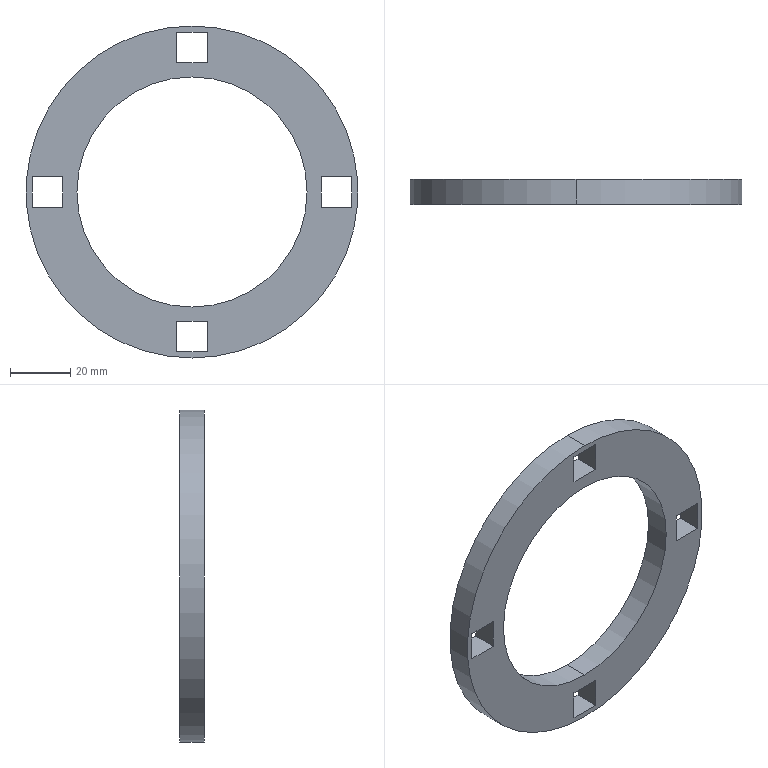Part | SolidWorks | features BaseBody 1 | 1 solid | 22 faces | box 110 x 8.25 x 110 mm | volume 37347 mm3 | plane 18 | cylinder 4 | commonest cylinder face diameters 76.25 x2 110 x2
STEP:
#1=CARTESIAN_POINT('',(-2080.019,753.694,-1572.562));
#2=VERTEX_POINT('',#1);
#3=CARTESIAN_POINT('',(-2090.144,753.694,-1572.562));
#4=VERTEX_POINT('',#3);
#5=CARTESIAN_POINT('',(-2080.019,753.694,-1572.562));
#6=DIRECTION('',(-1.,0.,0.));
#7=VECTOR('',#6,1000.);
#8=LINE('',#5,#7);
#9=EDGE_CURVE('',#2,#4,#8,.T.);
#10=ORIENTED_EDGE('',*,*,#9,.T.);
#11=CARTESIAN_POINT('',(-2090.144,753.694,-1582.687));
#12=VERTEX_POINT('',#11);
#13=CARTESIAN_POINT('',(-2090.144,753.694,-1572.562));
#14=DIRECTION('',(0.,0.,-1.));
#15=VECTOR('',#14,1000.);
#16=LINE('',#13,#15);
#17=EDGE_CURVE('',#4,#12,#16,.T.);
#18=ORIENTED_EDGE('',*,*,#17,.T.);
#19=CARTESIAN_POINT('',(-2080.019,753.694,-1582.687));
#20=VERTEX_POINT('',#19);
#21=CARTESIAN_POINT('',(-2090.144,753.694,-1582.687));
#22=DIRECTION('',(1.,0.,0.));
#23=VECTOR('',#22,1000.);
#24=LINE('',#21,#23);
#25=EDGE_CURVE('',#12,#20,#24,.T.);
#26=ORIENTED_EDGE('',*,*,#25,.T.);
#27=CARTESIAN_POINT('',(-2080.019,753.694,-1582.687));
#28=DIRECTION('',(0.,0.,1.));
#29=VECTOR('',#28,1000.);
#30=LINE('',#27,#29);
#31=EDGE_CURVE('',#20,#2,#30,.T.);
#32=ORIENTED_EDGE('',*,*,#31,.T.);
#33=EDGE_LOOP('',(#10,#18,#26,#32));
#34=FACE_BOUND('',#33,.T.);
#35=CARTESIAN_POINT('',(-2138.012,753.694,-1524.694));
#36=VERTEX_POINT('',#35);
#37=CARTESIAN_POINT('',(-2138.012,753.694,-1534.819));
#38=VERTEX_POINT('',#37);
#39=CARTESIAN_POINT('',(-2138.012,753.694,-1524.694));
#40=DIRECTION('',(0.,0.,-1.));
#41=VECTOR('',#40,1000.);
#42=LINE('',#39,#41);
#43=EDGE_CURVE('',#36,#38,#42,.T.);
#44=ORIENTED_EDGE('',*,*,#43,.T.);
#45=CARTESIAN_POINT('',(-2127.887,753.694,-1534.819));
#46=VERTEX_POINT('',#45);
#47=CARTESIAN_POINT('',(-2138.012,753.694,-1534.819));
#48=DIRECTION('',(1.,0.,0.));
#49=VECTOR('',#48,1000.);
#50=LINE('',#47,#49);
#51=EDGE_CURVE('',#38,#46,#50,.T.);
#52=ORIENTED_EDGE('',*,*,#51,.T.);
#53=CARTESIAN_POINT('',(-2127.887,753.694,-1524.694));
#54=VERTEX_POINT('',#53);
#55=CARTESIAN_POINT('',(-2127.887,753.694,-1534.819));
#56=DIRECTION('',(0.,0.,1.));
#57=VECTOR('',#56,1000.);
#58=LINE('',#55,#57);
#59=EDGE_CURVE('',#46,#54,#58,.T.);
#60=ORIENTED_EDGE('',*,*,#59,.T.);
#61=CARTESIAN_POINT('',(-2127.887,753.694,-1524.694));
#62=DIRECTION('',(-1.,0.,0.));
#63=VECTOR('',#62,1000.);
#64=LINE('',#61,#63);
#65=EDGE_CURVE('',#54,#36,#64,.T.);
#66=ORIENTED_EDGE('',*,*,#65,.T.);
#67=EDGE_LOOP('',(#44,#52,#60,#66));
#68=FACE_BOUND('',#67,.T.);
#69=CARTESIAN_POINT('',(-2185.88,753.694,-1582.687));
#70=VERTEX_POINT('',#69);
#71=CARTESIAN_POINT('',(-2175.755,753.694,-1582.687));
#72=VERTEX_POINT('',#71);
#73=CARTESIAN_POINT('',(-2185.88,753.694,-1582.687));
#74=DIRECTION('',(1.,0.,0.));
#75=VECTOR('',#74,1000.);
#76=LINE('',#73,#75);
#77=EDGE_CURVE('',#70,#72,#76,.T.);
#78=ORIENTED_EDGE('',*,*,#77,.T.);
#79=CARTESIAN_POINT('',(-2175.755,753.694,-1572.562));
#80=VERTEX_POINT('',#79);
#81=CARTESIAN_POINT('',(-2175.755,753.694,-1582.687));
#82=DIRECTION('',(0.,0.,1.));
#83=VECTOR('',#82,1000.);
#84=LINE('',#81,#83);
#85=EDGE_CURVE('',#72,#80,#84,.T.);
#86=ORIENTED_EDGE('',*,*,#85,.T.);
#87=CARTESIAN_POINT('',(-2185.88,753.694,-1572.562));
#88=VERTEX_POINT('',#87);
#89=CARTESIAN_POINT('',(-2175.755,753.694,-1572.562));
#90=DIRECTION('',(-1.,0.,0.));
#91=VECTOR('',#90,1000.);
#92=LINE('',#89,#91);
#93=EDGE_CURVE('',#80,#88,#92,.T.);
#94=ORIENTED_EDGE('',*,*,#93,.T.);
#95=CARTESIAN_POINT('',(-2185.88,753.694,-1572.562));
#96=DIRECTION('',(0.,0.,-1.));
#97=VECTOR('',#96,1000.);
#98=LINE('',#95,#97);
#99=EDGE_CURVE('',#88,#70,#98,.T.);
#100=ORIENTED_EDGE('',*,*,#99,.T.);
#101=EDGE_LOOP('',(#78,#86,#94,#100));
#102=FACE_BOUND('',#101,.T.);
#103=CARTESIAN_POINT('',(-2127.887,753.694,-1630.555));
#104=VERTEX_POINT('',#103);
#105=CARTESIAN_POINT('',(-2127.887,753.694,-1620.43));
#106=VERTEX_POINT('',#105);
#107=CARTESIAN_POINT('',(-2127.887,753.694,-1630.555));
#108=DIRECTION('',(0.,0.,1.));
#109=VECTOR('',#108,1000.);
#110=LINE('',#107,#109);
#111=EDGE_CURVE('',#104,#106,#110,.T.);
#112=ORIENTED_EDGE('',*,*,#111,.T.);
#113=CARTESIAN_POINT('',(-2138.012,753.694,-1620.43));
#114=VERTEX_POINT('',#113);
#115=CARTESIAN_POINT('',(-2127.887,753.694,-1620.43));
#116=DIRECTION('',(-1.,0.,0.));
#117=VECTOR('',#116,1000.);
#118=LINE('',#115,#117);
#119=EDGE_CURVE('',#106,#114,#118,.T.);
#120=ORIENTED_EDGE('',*,*,#119,.T.);
#121=CARTESIAN_POINT('',(-2138.012,753.694,-1630.555));
#122=VERTEX_POINT('',#121);
#123=CARTESIAN_POINT('',(-2138.012,753.694,-1620.43));
#124=DIRECTION('',(0.,0.,-1.));
#125=VECTOR('',#124,1000.);
#126=LINE('',#123,#125);
#127=EDGE_CURVE('',#114,#122,#126,.T.);
#128=ORIENTED_EDGE('',*,*,#127,.T.);
#129=CARTESIAN_POINT('',(-2138.012,753.694,-1630.555));
#130=DIRECTION('',(1.,0.,0.));
#131=VECTOR('',#130,1000.);
#132=LINE('',#129,#131);
#133=EDGE_CURVE('',#122,#104,#132,.T.);
#134=ORIENTED_EDGE('',*,*,#133,.T.);
#135=EDGE_LOOP('',(#112,#120,#128,#134));
#136=FACE_BOUND('',#135,.T.);
#137=CARTESIAN_POINT('',(-2132.95,753.694,-1539.499));
#138=VERTEX_POINT('',#137);
#139=CARTESIAN_POINT('',(-2132.95,753.694,-1615.749));
#140=VERTEX_POINT('',#139);
#141=CARTESIAN_POINT('',(-2132.95,753.694,-1577.624));
#142=DIRECTION('',(0.,1.,0.));
#143=DIRECTION('',(0.,0.,1.));
#144=AXIS2_PLACEMENT_3D('',#141,#142,#143);
#145=CIRCLE('',#144,38.125);
#146=EDGE_CURVE('',#138,#140,#145,.T.);
#147=ORIENTED_EDGE('',*,*,#146,.F.);
#148=CARTESIAN_POINT('',(-2132.95,753.694,-1577.624));
#149=DIRECTION('',(0.,1.,0.));
#150=DIRECTION('',(0.,0.,-1.));
#151=AXIS2_PLACEMENT_3D('',#148,#149,#150);
#152=CIRCLE('',#151,38.125);
#153=EDGE_CURVE('',#140,#138,#152,.T.);
#154=ORIENTED_EDGE('',*,*,#153,.F.);
#155=EDGE_LOOP('',(#147,#154));
#156=FACE_BOUND('',#155,.T.);
#157=CARTESIAN_POINT('',(-2132.95,753.694,-1632.624));
#158=VERTEX_POINT('',#157);
#159=CARTESIAN_POINT('',(-2132.95,753.694,-1522.624));
#160=VERTEX_POINT('',#159);
#161=CARTESIAN_POINT('',(-2132.95,753.694,-1577.624));
#162=DIRECTION('',(0.,1.,0.));
#163=DIRECTION('',(0.,0.,-1.));
#164=AXIS2_PLACEMENT_3D('',#161,#162,#163);
#165=CIRCLE('',#164,55.);
#166=EDGE_CURVE('',#158,#160,#165,.T.);
#167=ORIENTED_EDGE('',*,*,#166,.T.);
#168=CARTESIAN_POINT('',(-2132.95,753.694,-1577.624));
#169=DIRECTION('',(0.,1.,0.));
#170=DIRECTION('',(0.,0.,1.));
#171=AXIS2_PLACEMENT_3D('',#168,#169,#170);
#172=CIRCLE('',#171,55.);
#173=EDGE_CURVE('',#160,#158,#172,.T.);
#174=ORIENTED_EDGE('',*,*,#173,.T.);
#175=EDGE_LOOP('',(#167,#174));
#176=FACE_OUTER_BOUND('',#175,.T.);
#177=CARTESIAN_POINT('',(-2072.49,753.694,-1517.124));
#178=DIRECTION('',(0.,1.,0.));
#179=DIRECTION('',(1.,0.,0.));
#180=AXIS2_PLACEMENT_3D('',#177,#178,#179);
#181=PLANE('',#180);
#182=ADVANCED_FACE('',(#34,#68,#102,#136,#156,#176),#181,.T.);
#183=CARTESIAN_POINT('',(-2090.144,745.444,-1572.562));
#184=VERTEX_POINT('',#183);
#185=CARTESIAN_POINT('',(-2080.019,745.444,-1572.562));
#186=VERTEX_POINT('',#185);
#187=CARTESIAN_POINT('',(-2090.144,745.444,-1572.562));
#188=DIRECTION('',(1.,0.,0.));
#189=VECTOR('',#188,1000.);
#190=LINE('',#187,#189);
#191=EDGE_CURVE('',#184,#186,#190,.T.);
#192=ORIENTED_EDGE('',*,*,#191,.T.);
#193=CARTESIAN_POINT('',(-2080.019,745.444,-1582.687));
#194=VERTEX_POINT('',#193);
#195=CARTESIAN_POINT('',(-2080.019,745.444,-1572.562));
#196=DIRECTION('',(0.,0.,-1.));
#197=VECTOR('',#196,1000.);
#198=LINE('',#195,#197);
#199=EDGE_CURVE('',#186,#194,#198,.T.);
#200=ORIENTED_EDGE('',*,*,#199,.T.);
#201=CARTESIAN_POINT('',(-2090.144,745.444,-1582.687));
#202=VERTEX_POINT('',#201);
#203=CARTESIAN_POINT('',(-2080.019,745.444,-1582.687));
#204=DIRECTION('',(-1.,0.,0.));
#205=VECTOR('',#204,1000.);
#206=LINE('',#203,#205);
#207=EDGE_CURVE('',#194,#202,#206,.T.);
#208=ORIENTED_EDGE('',*,*,#207,.T.);
#209=CARTESIAN_POINT('',(-2090.144,745.444,-1582.687));
#210=DIRECTION('',(0.,0.,1.));
#211=VECTOR('',#210,1000.);
#212=LINE('',#209,#211);
#213=EDGE_CURVE('',#202,#184,#212,.T.);
#214=ORIENTED_EDGE('',*,*,#213,.T.);
#215=EDGE_LOOP('',(#192,#200,#208,#214));
#216=FACE_BOUND('',#215,.T.);
#217=CARTESIAN_POINT('',(-2138.012,745.444,-1534.819));
#218=VERTEX_POINT('',#217);
#219=CARTESIAN_POINT('',(-2138.012,745.444,-1524.694));
#220=VERTEX_POINT('',#219);
#221=CARTESIAN_POINT('',(-2138.012,745.444,-1534.819));
#222=DIRECTION('',(0.,0.,1.));
#223=VECTOR('',#222,1000.);
#224=LINE('',#221,#223);
#225=EDGE_CURVE('',#218,#220,#224,.T.);
#226=ORIENTED_EDGE('',*,*,#225,.T.);
#227=CARTESIAN_POINT('',(-2127.887,745.444,-1524.694));
#228=VERTEX_POINT('',#227);
#229=CARTESIAN_POINT('',(-2138.012,745.444,-1524.694));
#230=DIRECTION('',(1.,0.,0.));
#231=VECTOR('',#230,1000.);
#232=LINE('',#229,#231);
#233=EDGE_CURVE('',#220,#228,#232,.T.);
#234=ORIENTED_EDGE('',*,*,#233,.T.);
#235=CARTESIAN_POINT('',(-2127.887,745.444,-1534.819));
#236=VERTEX_POINT('',#235);
#237=CARTESIAN_POINT('',(-2127.887,745.444,-1524.694));
#238=DIRECTION('',(0.,0.,-1.));
#239=VECTOR('',#238,1000.);
#240=LINE('',#237,#239);
#241=EDGE_CURVE('',#228,#236,#240,.T.);
#242=ORIENTED_EDGE('',*,*,#241,.T.);
#243=CARTESIAN_POINT('',(-2127.887,745.444,-1534.819));
#244=DIRECTION('',(-1.,0.,0.));
#245=VECTOR('',#244,1000.);
#246=LINE('',#243,#245);
#247=EDGE_CURVE('',#236,#218,#246,.T.);
#248=ORIENTED_EDGE('',*,*,#247,.T.);
#249=EDGE_LOOP('',(#226,#234,#242,#248));
#250=FACE_BOUND('',#249,.T.);
#251=CARTESIAN_POINT('',(-2175.755,745.444,-1582.687));
#252=VERTEX_POINT('',#251);
#253=CARTESIAN_POINT('',(-2185.88,745.444,-1582.687));
#254=VERTEX_POINT('',#253);
#255=CARTESIAN_POINT('',(-2175.755,745.444,-1582.687));
#256=DIRECTION('',(-1.,0.,0.));
#257=VECTOR('',#256,1000.);
#258=LINE('',#255,#257);
#259=EDGE_CURVE('',#252,#254,#258,.T.);
#260=ORIENTED_EDGE('',*,*,#259,.T.);
#261=CARTESIAN_POINT('',(-2185.88,745.444,-1572.562));
#262=VERTEX_POINT('',#261);
#263=CARTESIAN_POINT('',(-2185.88,745.444,-1582.687));
#264=DIRECTION('',(0.,0.,1.));
#265=VECTOR('',#264,1000.);
#266=LINE('',#263,#265);
#267=EDGE_CURVE('',#254,#262,#266,.T.);
#268=ORIENTED_EDGE('',*,*,#267,.T.);
#269=CARTESIAN_POINT('',(-2175.755,745.444,-1572.562));
#270=VERTEX_POINT('',#269);
#271=CARTESIAN_POINT('',(-2185.88,745.444,-1572.562));
#272=DIRECTION('',(1.,0.,0.));
#273=VECTOR('',#272,1000.);
#274=LINE('',#271,#273);
#275=EDGE_CURVE('',#262,#270,#274,.T.);
#276=ORIENTED_EDGE('',*,*,#275,.T.);
#277=CARTESIAN_POINT('',(-2175.755,745.444,-1572.562));
#278=DIRECTION('',(0.,0.,-1.));
#279=VECTOR('',#278,1000.);
#280=LINE('',#277,#279);
#281=EDGE_CURVE('',#270,#252,#280,.T.);
#282=ORIENTED_EDGE('',*,*,#281,.T.);
#283=EDGE_LOOP('',(#260,#268,#276,#282));
#284=FACE_BOUND('',#283,.T.);
#285=CARTESIAN_POINT('',(-2127.887,745.444,-1620.43));
#286=VERTEX_POINT('',#285);
#287=CARTESIAN_POINT('',(-2127.887,745.444,-1630.555));
#288=VERTEX_POINT('',#287);
#289=CARTESIAN_POINT('',(-2127.887,745.444,-1620.43));
#290=DIRECTION('',(0.,0.,-1.));
#291=VECTOR('',#290,1000.);
#292=LINE('',#289,#291);
#293=EDGE_CURVE('',#286,#288,#292,.T.);
#294=ORIENTED_EDGE('',*,*,#293,.T.);
#295=CARTESIAN_POINT('',(-2138.012,745.444,-1630.555));
#296=VERTEX_POINT('',#295);
#297=CARTESIAN_POINT('',(-2127.887,745.444,-1630.555));
#298=DIRECTION('',(-1.,0.,0.));
#299=VECTOR('',#298,1000.);
#300=LINE('',#297,#299);
#301=EDGE_CURVE('',#288,#296,#300,.T.);
#302=ORIENTED_EDGE('',*,*,#301,.T.);
#303=CARTESIAN_POINT('',(-2138.012,745.444,-1620.43));
#304=VERTEX_POINT('',#303);
#305=CARTESIAN_POINT('',(-2138.012,745.444,-1630.555));
#306=DIRECTION('',(0.,0.,1.));
#307=VECTOR('',#306,1000.);
#308=LINE('',#305,#307);
#309=EDGE_CURVE('',#296,#304,#308,.T.);
#310=ORIENTED_EDGE('',*,*,#309,.T.);
#311=CARTESIAN_POINT('',(-2138.012,745.444,-1620.43));
#312=DIRECTION('',(1.,0.,0.));
#313=VECTOR('',#312,1000.);
#314=LINE('',#311,#313);
#315=EDGE_CURVE('',#304,#286,#314,.T.);
#316=ORIENTED_EDGE('',*,*,#315,.T.);
#317=EDGE_LOOP('',(#294,#302,#310,#316));
#318=FACE_BOUND('',#317,.T.);
#319=CARTESIAN_POINT('',(-2132.95,745.444,-1539.499));
#320=VERTEX_POINT('',#319);
#321=CARTESIAN_POINT('',(-2132.95,745.444,-1615.749));
#322=VERTEX_POINT('',#321);
#323=CARTESIAN_POINT('',(-2132.95,745.444,-1577.624));
#324=DIRECTION('',(0.,-1.,0.));
#325=DIRECTION('',(0.,0.,1.));
#326=AXIS2_PLACEMENT_3D('',#323,#324,#325);
#327=CIRCLE('',#326,38.125);
#328=EDGE_CURVE('',#320,#322,#327,.T.);
#329=ORIENTED_EDGE('',*,*,#328,.F.);
#330=CARTESIAN_POINT('',(-2132.95,745.444,-1577.624));
#331=DIRECTION('',(0.,-1.,0.));
#332=DIRECTION('',(0.,0.,-1.));
#333=AXIS2_PLACEMENT_3D('',#330,#331,#332);
#334=CIRCLE('',#333,38.125);
#335=EDGE_CURVE('',#322,#320,#334,.T.);
#336=ORIENTED_EDGE('',*,*,#335,.F.);
#337=EDGE_LOOP('',(#329,#336));
#338=FACE_BOUND('',#337,.T.);
#339=CARTESIAN_POINT('',(-2132.95,745.444,-1632.624));
#340=VERTEX_POINT('',#339);
#341=CARTESIAN_POINT('',(-2132.95,745.444,-1522.624));
#342=VERTEX_POINT('',#341);
#343=CARTESIAN_POINT('',(-2132.95,745.444,-1577.624));
#344=DIRECTION('',(0.,-1.,0.));
#345=DIRECTION('',(0.,0.,-1.));
#346=AXIS2_PLACEMENT_3D('',#343,#344,#345);
#347=CIRCLE('',#346,55.);
#348=EDGE_CURVE('',#340,#342,#347,.T.);
#349=ORIENTED_EDGE('',*,*,#348,.T.);
#350=CARTESIAN_POINT('',(-2132.95,745.444,-1577.624));
#351=DIRECTION('',(0.,-1.,0.));
#352=DIRECTION('',(0.,0.,1.));
#353=AXIS2_PLACEMENT_3D('',#350,#351,#352);
#354=CIRCLE('',#353,55.);
#355=EDGE_CURVE('',#342,#340,#354,.T.);
#356=ORIENTED_EDGE('',*,*,#355,.T.);
#357=EDGE_LOOP('',(#349,#356));
#358=FACE_OUTER_BOUND('',#357,.T.);
#359=CARTESIAN_POINT('',(-2072.49,745.444,-1638.124));
#360=DIRECTION('',(0.,-1.,0.));
#361=DIRECTION('',(0.,0.,-1.));
#362=AXIS2_PLACEMENT_3D('',#359,#360,#361);
#363=PLANE('',#362);
#364=ADVANCED_FACE('',(#216,#250,#284,#318,#338,#358),#363,.T.);
#365=CARTESIAN_POINT('',(-2132.95,745.444,-1632.624));
#366=DIRECTION('',(0.,1.,0.));
#367=VECTOR('',#366,1000.);
#368=LINE('',#365,#367);
#369=EDGE_CURVE('',#340,#158,#368,.T.);
#370=ORIENTED_EDGE('',*,*,#369,.T.);
#371=ORIENTED_EDGE('',*,*,#173,.F.);
#372=CARTESIAN_POINT('',(-2132.95,753.694,-1522.624));
#373=DIRECTION('',(0.,-1.,0.));
#374=VECTOR('',#373,1000.);
#375=LINE('',#372,#374);
#376=EDGE_CURVE('',#160,#342,#375,.T.);
#377=ORIENTED_EDGE('',*,*,#376,.T.);
#378=ORIENTED_EDGE('',*,*,#348,.F.);
#379=EDGE_LOOP('',(#370,#371,#377,#378));
#380=FACE_OUTER_BOUND('',#379,.T.);
#381=CARTESIAN_POINT('',(-2132.95,745.031,-1577.624));
#382=DIRECTION('',(0.,-1.,0.));
#383=DIRECTION('',(-0.08716,0.,-0.9962));
#384=AXIS2_PLACEMENT_3D('',#381,#382,#383);
#385=CYLINDRICAL_SURFACE('',#384,55.);
#386=ADVANCED_FACE('',(#380),#385,.T.);
#387=CARTESIAN_POINT('',(-2132.95,753.694,-1615.749));
#388=DIRECTION('',(0.,-1.,0.));
#389=VECTOR('',#388,1000.);
#390=LINE('',#387,#389);
#391=EDGE_CURVE('',#140,#322,#390,.T.);
#392=ORIENTED_EDGE('',*,*,#391,.T.);
#393=ORIENTED_EDGE('',*,*,#335,.T.);
#394=CARTESIAN_POINT('',(-2132.95,745.444,-1539.499));
#395=DIRECTION('',(0.,1.,0.));
#396=VECTOR('',#395,1000.);
#397=LINE('',#394,#396);
#398=EDGE_CURVE('',#320,#138,#397,.T.);
#399=ORIENTED_EDGE('',*,*,#398,.T.);
#400=ORIENTED_EDGE('',*,*,#146,.T.);
#401=EDGE_LOOP('',(#392,#393,#399,#400));
#402=FACE_OUTER_BOUND('',#401,.T.);
#403=CARTESIAN_POINT('',(-2132.95,754.106,-1577.624));
#404=DIRECTION('',(0.,-1.,0.));
#405=DIRECTION('',(-0.08716,0.,-0.9962));
#406=AXIS2_PLACEMENT_3D('',#403,#404,#405);
#407=CYLINDRICAL_SURFACE('',#406,38.125);
#408=ADVANCED_FACE('',(#402),#407,.F.);
#409=ORIENTED_EDGE('',*,*,#301,.F.);
#410=CARTESIAN_POINT('',(-2127.887,753.694,-1630.555));
#411=DIRECTION('',(0.,-1.,0.));
#412=VECTOR('',#411,1000.);
#413=LINE('',#410,#412);
#414=EDGE_CURVE('',#104,#288,#413,.T.);
#415=ORIENTED_EDGE('',*,*,#414,.F.);
#416=ORIENTED_EDGE('',*,*,#133,.F.);
#417=CARTESIAN_POINT('',(-2138.012,753.694,-1630.555));
#418=DIRECTION('',(0.,-1.,0.));
#419=VECTOR('',#418,1000.);
#420=LINE('',#417,#419);
#421=EDGE_CURVE('',#122,#296,#420,.T.);
#422=ORIENTED_EDGE('',*,*,#421,.T.);
#423=EDGE_LOOP('',(#409,#415,#416,#422));
#424=FACE_OUTER_BOUND('',#423,.T.);
#425=CARTESIAN_POINT('',(-2127.381,744.937,-1630.555));
#426=DIRECTION('',(0.,0.,1.));
#427=DIRECTION('',(1.,0.,0.));
#428=AXIS2_PLACEMENT_3D('',#425,#426,#427);
#429=PLANE('',#428);
#430=ADVANCED_FACE('',(#424),#429,.T.);
#431=ORIENTED_EDGE('',*,*,#293,.F.);
#432=CARTESIAN_POINT('',(-2127.887,753.694,-1620.43));
#433=DIRECTION('',(0.,-1.,0.));
#434=VECTOR('',#433,1000.);
#435=LINE('',#432,#434);
#436=EDGE_CURVE('',#106,#286,#435,.T.);
#437=ORIENTED_EDGE('',*,*,#436,.F.);
#438=ORIENTED_EDGE('',*,*,#111,.F.);
#439=ORIENTED_EDGE('',*,*,#414,.T.);
#440=EDGE_LOOP('',(#431,#437,#438,#439));
#441=FACE_OUTER_BOUND('',#440,.T.);
#442=CARTESIAN_POINT('',(-2127.887,744.937,-1619.924));
#443=DIRECTION('',(-1.,0.,0.));
#444=DIRECTION('',(0.,0.,1.));
#445=AXIS2_PLACEMENT_3D('',#442,#443,#444);
#446=PLANE('',#445);
#447=ADVANCED_FACE('',(#441),#446,.T.);
#448=ORIENTED_EDGE('',*,*,#315,.F.);
#449=CARTESIAN_POINT('',(-2138.012,753.694,-1620.43));
#450=DIRECTION('',(0.,-1.,0.));
#451=VECTOR('',#450,1000.);
#452=LINE('',#449,#451);
#453=EDGE_CURVE('',#114,#304,#452,.T.);
#454=ORIENTED_EDGE('',*,*,#453,.F.);
#455=ORIENTED_EDGE('',*,*,#119,.F.);
#456=ORIENTED_EDGE('',*,*,#436,.T.);
#457=EDGE_LOOP('',(#448,#454,#455,#456));
#458=FACE_OUTER_BOUND('',#457,.T.);
#459=CARTESIAN_POINT('',(-2127.381,754.2,-1620.43));
#460=DIRECTION('',(0.,0.,-1.));
#461=DIRECTION('',(0.,-1.,0.));
#462=AXIS2_PLACEMENT_3D('',#459,#460,#461);
#463=PLANE('',#462);
#464=ADVANCED_FACE('',(#458),#463,.T.);
#465=ORIENTED_EDGE('',*,*,#309,.F.);
#466=ORIENTED_EDGE('',*,*,#421,.F.);
#467=ORIENTED_EDGE('',*,*,#127,.F.);
#468=ORIENTED_EDGE('',*,*,#453,.T.);
#469=EDGE_LOOP('',(#465,#466,#467,#468));
#470=FACE_OUTER_BOUND('',#469,.T.);
#471=CARTESIAN_POINT('',(-2138.012,754.2,-1619.924));
#472=DIRECTION('',(1.,0.,0.));
#473=DIRECTION('',(0.,1.,0.));
#474=AXIS2_PLACEMENT_3D('',#471,#472,#473);
#475=PLANE('',#474);
#476=ADVANCED_FACE('',(#470),#475,.T.);
#477=ORIENTED_EDGE('',*,*,#267,.F.);
#478=CARTESIAN_POINT('',(-2185.88,753.694,-1582.687));
#479=DIRECTION('',(0.,-1.,0.));
#480=VECTOR('',#479,1000.);
#481=LINE('',#478,#480);
#482=EDGE_CURVE('',#70,#254,#481,.T.);
#483=ORIENTED_EDGE('',*,*,#482,.F.);
#484=ORIENTED_EDGE('',*,*,#99,.F.);
#485=CARTESIAN_POINT('',(-2185.88,753.694,-1572.562));
#486=DIRECTION('',(0.,-1.,0.));
#487=VECTOR('',#486,1000.);
#488=LINE('',#485,#487);
#489=EDGE_CURVE('',#88,#262,#488,.T.);
#490=ORIENTED_EDGE('',*,*,#489,.T.);
#491=EDGE_LOOP('',(#477,#483,#484,#490));
#492=FACE_OUTER_BOUND('',#491,.T.);
#493=CARTESIAN_POINT('',(-2185.88,744.937,-1583.193));
#494=DIRECTION('',(1.,0.,0.));
#495=DIRECTION('',(0.,1.,0.));
#496=AXIS2_PLACEMENT_3D('',#493,#494,#495);
#497=PLANE('',#496);
#498=ADVANCED_FACE('',(#492),#497,.T.);
#499=ORIENTED_EDGE('',*,*,#259,.F.);
#500=CARTESIAN_POINT('',(-2175.755,753.694,-1582.687));
#501=DIRECTION('',(0.,-1.,0.));
#502=VECTOR('',#501,1000.);
#503=LINE('',#500,#502);
#504=EDGE_CURVE('',#72,#252,#503,.T.);
#505=ORIENTED_EDGE('',*,*,#504,.F.);
#506=ORIENTED_EDGE('',*,*,#77,.F.);
#507=ORIENTED_EDGE('',*,*,#482,.T.);
#508=EDGE_LOOP('',(#499,#505,#506,#507));
#509=FACE_OUTER_BOUND('',#508,.T.);
#510=CARTESIAN_POINT('',(-2175.249,744.937,-1582.687));
#511=DIRECTION('',(0.,0.,1.));
#512=DIRECTION('',(1.,0.,0.));
#513=AXIS2_PLACEMENT_3D('',#510,#511,#512);
#514=PLANE('',#513);
#515=ADVANCED_FACE('',(#509),#514,.T.);
#516=ORIENTED_EDGE('',*,*,#281,.F.);
#517=CARTESIAN_POINT('',(-2175.755,753.694,-1572.562));
#518=DIRECTION('',(0.,-1.,0.));
#519=VECTOR('',#518,1000.);
#520=LINE('',#517,#519);
#521=EDGE_CURVE('',#80,#270,#520,.T.);
#522=ORIENTED_EDGE('',*,*,#521,.F.);
#523=ORIENTED_EDGE('',*,*,#85,.F.);
#524=ORIENTED_EDGE('',*,*,#504,.T.);
#525=EDGE_LOOP('',(#516,#522,#523,#524));
#526=FACE_OUTER_BOUND('',#525,.T.);
#527=CARTESIAN_POINT('',(-2175.755,754.2,-1583.193));
#528=DIRECTION('',(-1.,0.,0.));
#529=DIRECTION('',(0.,0.,1.));
#530=AXIS2_PLACEMENT_3D('',#527,#528,#529);
#531=PLANE('',#530);
#532=ADVANCED_FACE('',(#526),#531,.T.);
#533=ORIENTED_EDGE('',*,*,#275,.F.);
#534=ORIENTED_EDGE('',*,*,#489,.F.);
#535=ORIENTED_EDGE('',*,*,#93,.F.);
#536=ORIENTED_EDGE('',*,*,#521,.T.);
#537=EDGE_LOOP('',(#533,#534,#535,#536));
#538=FACE_OUTER_BOUND('',#537,.T.);
#539=CARTESIAN_POINT('',(-2175.249,754.2,-1572.562));
#540=DIRECTION('',(0.,0.,-1.));
#541=DIRECTION('',(0.,-1.,0.));
#542=AXIS2_PLACEMENT_3D('',#539,#540,#541);
#543=PLANE('',#542);
#544=ADVANCED_FACE('',(#538),#543,.T.);
#545=ORIENTED_EDGE('',*,*,#233,.F.);
#546=CARTESIAN_POINT('',(-2138.012,753.694,-1524.694));
#547=DIRECTION('',(0.,-1.,0.));
#548=VECTOR('',#547,1000.);
#549=LINE('',#546,#548);
#550=EDGE_CURVE('',#36,#220,#549,.T.);
#551=ORIENTED_EDGE('',*,*,#550,.F.);
#552=ORIENTED_EDGE('',*,*,#65,.F.);
#553=CARTESIAN_POINT('',(-2127.887,753.694,-1524.694));
#554=DIRECTION('',(0.,-1.,0.));
#555=VECTOR('',#554,1000.);
#556=LINE('',#553,#555);
#557=EDGE_CURVE('',#54,#228,#556,.T.);
#558=ORIENTED_EDGE('',*,*,#557,.T.);
#559=EDGE_LOOP('',(#545,#551,#552,#558));
#560=FACE_OUTER_BOUND('',#559,.T.);
#561=CARTESIAN_POINT('',(-2138.518,744.937,-1524.694));
#562=DIRECTION('',(0.,0.,-1.));
#563=DIRECTION('',(0.,-1.,0.));
#564=AXIS2_PLACEMENT_3D('',#561,#562,#563);
#565=PLANE('',#564);
#566=ADVANCED_FACE('',(#560),#565,.T.);
#567=ORIENTED_EDGE('',*,*,#225,.F.);
#568=CARTESIAN_POINT('',(-2138.012,753.694,-1534.819));
#569=DIRECTION('',(0.,-1.,0.));
#570=VECTOR('',#569,1000.);
#571=LINE('',#568,#570);
#572=EDGE_CURVE('',#38,#218,#571,.T.);
#573=ORIENTED_EDGE('',*,*,#572,.F.);
#574=ORIENTED_EDGE('',*,*,#43,.F.);
#575=ORIENTED_EDGE('',*,*,#550,.T.);
#576=EDGE_LOOP('',(#567,#573,#574,#575));
#577=FACE_OUTER_BOUND('',#576,.T.);
#578=CARTESIAN_POINT('',(-2138.012,744.937,-1535.325));
#579=DIRECTION('',(1.,0.,0.));
#580=DIRECTION('',(0.,1.,0.));
#581=AXIS2_PLACEMENT_3D('',#578,#579,#580);
#582=PLANE('',#581);
#583=ADVANCED_FACE('',(#577),#582,.T.);
#584=ORIENTED_EDGE('',*,*,#247,.F.);
#585=CARTESIAN_POINT('',(-2127.887,753.694,-1534.819));
#586=DIRECTION('',(0.,-1.,0.));
#587=VECTOR('',#586,1000.);
#588=LINE('',#585,#587);
#589=EDGE_CURVE('',#46,#236,#588,.T.);
#590=ORIENTED_EDGE('',*,*,#589,.F.);
#591=ORIENTED_EDGE('',*,*,#51,.F.);
#592=ORIENTED_EDGE('',*,*,#572,.T.);
#593=EDGE_LOOP('',(#584,#590,#591,#592));
#594=FACE_OUTER_BOUND('',#593,.T.);
#595=CARTESIAN_POINT('',(-2138.518,754.2,-1534.819));
#596=DIRECTION('',(0.,0.,1.));
#597=DIRECTION('',(1.,0.,0.));
#598=AXIS2_PLACEMENT_3D('',#595,#596,#597);
#599=PLANE('',#598);
#600=ADVANCED_FACE('',(#594),#599,.T.);
#601=ORIENTED_EDGE('',*,*,#241,.F.);
#602=ORIENTED_EDGE('',*,*,#557,.F.);
#603=ORIENTED_EDGE('',*,*,#59,.F.);
#604=ORIENTED_EDGE('',*,*,#589,.T.);
#605=EDGE_LOOP('',(#601,#602,#603,#604));
#606=FACE_OUTER_BOUND('',#605,.T.);
#607=CARTESIAN_POINT('',(-2127.887,754.2,-1535.325));
#608=DIRECTION('',(-1.,0.,0.));
#609=DIRECTION('',(0.,0.,1.));
#610=AXIS2_PLACEMENT_3D('',#607,#608,#609);
#611=PLANE('',#610);
#612=ADVANCED_FACE('',(#606),#611,.T.);
#613=ORIENTED_EDGE('',*,*,#199,.F.);
#614=CARTESIAN_POINT('',(-2080.019,753.694,-1572.562));
#615=DIRECTION('',(0.,-1.,0.));
#616=VECTOR('',#615,1000.);
#617=LINE('',#614,#616);
#618=EDGE_CURVE('',#2,#186,#617,.T.);
#619=ORIENTED_EDGE('',*,*,#618,.F.);
#620=ORIENTED_EDGE('',*,*,#31,.F.);
#621=CARTESIAN_POINT('',(-2080.019,753.694,-1582.687));
#622=DIRECTION('',(0.,-1.,0.));
#623=VECTOR('',#622,1000.);
#624=LINE('',#621,#623);
#625=EDGE_CURVE('',#20,#194,#624,.T.);
#626=ORIENTED_EDGE('',*,*,#625,.T.);
#627=EDGE_LOOP('',(#613,#619,#620,#626));
#628=FACE_OUTER_BOUND('',#627,.T.);
#629=CARTESIAN_POINT('',(-2080.019,744.937,-1572.056));
#630=DIRECTION('',(-1.,0.,0.));
#631=DIRECTION('',(0.,0.,1.));
#632=AXIS2_PLACEMENT_3D('',#629,#630,#631);
#633=PLANE('',#632);
#634=ADVANCED_FACE('',(#628),#633,.T.);
#635=ORIENTED_EDGE('',*,*,#191,.F.);
#636=CARTESIAN_POINT('',(-2090.144,753.694,-1572.562));
#637=DIRECTION('',(0.,-1.,0.));
#638=VECTOR('',#637,1000.);
#639=LINE('',#636,#638);
#640=EDGE_CURVE('',#4,#184,#639,.T.);
#641=ORIENTED_EDGE('',*,*,#640,.F.);
#642=ORIENTED_EDGE('',*,*,#9,.F.);
#643=ORIENTED_EDGE('',*,*,#618,.T.);
#644=EDGE_LOOP('',(#635,#641,#642,#643));
#645=FACE_OUTER_BOUND('',#644,.T.);
#646=CARTESIAN_POINT('',(-2090.65,744.937,-1572.562));
#647=DIRECTION('',(0.,0.,-1.));
#648=DIRECTION('',(0.,-1.,0.));
#649=AXIS2_PLACEMENT_3D('',#646,#647,#648);
#650=PLANE('',#649);
#651=ADVANCED_FACE('',(#645),#650,.T.);
#652=ORIENTED_EDGE('',*,*,#213,.F.);
#653=CARTESIAN_POINT('',(-2090.144,753.694,-1582.687));
#654=DIRECTION('',(0.,-1.,0.));
#655=VECTOR('',#654,1000.);
#656=LINE('',#653,#655);
#657=EDGE_CURVE('',#12,#202,#656,.T.);
#658=ORIENTED_EDGE('',*,*,#657,.F.);
#659=ORIENTED_EDGE('',*,*,#17,.F.);
#660=ORIENTED_EDGE('',*,*,#640,.T.);
#661=EDGE_LOOP('',(#652,#658,#659,#660));
#662=FACE_OUTER_BOUND('',#661,.T.);
#663=CARTESIAN_POINT('',(-2090.144,754.2,-1572.056));
#664=DIRECTION('',(1.,0.,0.));
#665=DIRECTION('',(0.,1.,0.));
#666=AXIS2_PLACEMENT_3D('',#663,#664,#665);
#667=PLANE('',#666);
#668=ADVANCED_FACE('',(#662),#667,.T.);
#669=ORIENTED_EDGE('',*,*,#207,.F.);
#670=ORIENTED_EDGE('',*,*,#625,.F.);
#671=ORIENTED_EDGE('',*,*,#25,.F.);
#672=ORIENTED_EDGE('',*,*,#657,.T.);
#673=EDGE_LOOP('',(#669,#670,#671,#672));
#674=FACE_OUTER_BOUND('',#673,.T.);
#675=CARTESIAN_POINT('',(-2090.65,754.2,-1582.687));
#676=DIRECTION('',(0.,0.,1.));
#677=DIRECTION('',(1.,0.,0.));
#678=AXIS2_PLACEMENT_3D('',#675,#676,#677);
#679=PLANE('',#678);
#680=ADVANCED_FACE('',(#674),#679,.T.);
#681=ORIENTED_EDGE('',*,*,#391,.F.);
#682=ORIENTED_EDGE('',*,*,#153,.T.);
#683=ORIENTED_EDGE('',*,*,#398,.F.);
#684=ORIENTED_EDGE('',*,*,#328,.T.);
#685=EDGE_LOOP('',(#681,#682,#683,#684));
#686=FACE_OUTER_BOUND('',#685,.T.);
#687=CARTESIAN_POINT('',(-2132.95,754.106,-1577.624));
#688=DIRECTION('',(0.,-1.,0.));
#689=DIRECTION('',(0.08716,0.,0.9962));
#690=AXIS2_PLACEMENT_3D('',#687,#688,#689);
#691=CYLINDRICAL_SURFACE('',#690,38.125);
#692=ADVANCED_FACE('',(#686),#691,.F.);
#693=ORIENTED_EDGE('',*,*,#369,.F.);
#694=ORIENTED_EDGE('',*,*,#355,.F.);
#695=ORIENTED_EDGE('',*,*,#376,.F.);
#696=ORIENTED_EDGE('',*,*,#166,.F.);
#697=EDGE_LOOP('',(#693,#694,#695,#696));
#698=FACE_OUTER_BOUND('',#697,.T.);
#699=CARTESIAN_POINT('',(-2132.95,745.031,-1577.624));
#700=DIRECTION('',(0.,-1.,0.));
#701=DIRECTION('',(0.08716,0.,0.9962));
#702=AXIS2_PLACEMENT_3D('',#699,#700,#701);
#703=CYLINDRICAL_SURFACE('',#702,55.);
#704=ADVANCED_FACE('',(#698),#703,.T.);
#705=CLOSED_SHELL('',(#182,#364,#386,#408,#430,#447,#464,#476,#498,#515,#532,#544,#566,#583,#600,#612,#634,#651,#668,#680,#692,#704));
#706=MANIFOLD_SOLID_BREP('',#705);
#707=CARTESIAN_POINT('',(0.,0.,0.));
#708=DIRECTION('',(0.,0.,1.));
#709=DIRECTION('',(1.,0.,0.));
#710=AXIS2_PLACEMENT_3D('',#707,#708,#709);
#711=(LENGTH_UNIT()NAMED_UNIT(*)SI_UNIT(.MILLI.,.METRE.));
#712=UNCERTAINTY_MEASURE_WITH_UNIT(LENGTH_MEASURE(0.00001),#711,'','');
#713=(NAMED_UNIT(*)PLANE_ANGLE_UNIT()SI_UNIT($,.RADIAN.));
#714=(NAMED_UNIT(*)SI_UNIT($,.STERADIAN.)SOLID_ANGLE_UNIT());
#715=(GEOMETRIC_REPRESENTATION_CONTEXT(3)GLOBAL_UNCERTAINTY_ASSIGNED_CONTEXT((#712))GLOBAL_UNIT_ASSIGNED_CONTEXT((#711,#713,#714))REPRESENTATION_CONTEXT('',''));
#716=ADVANCED_BREP_SHAPE_REPRESENTATION('',(#706,#710),#715);